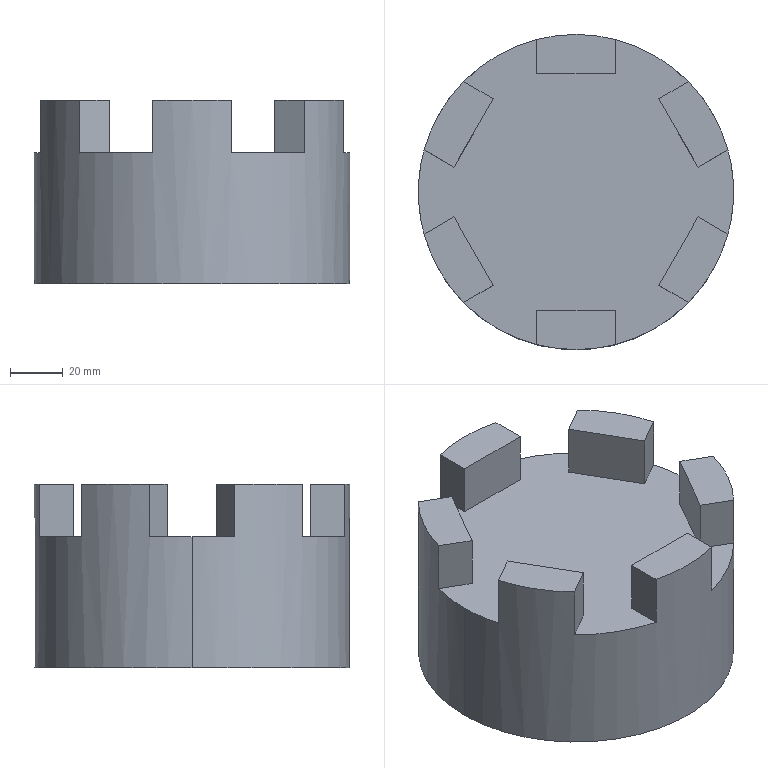Part | SolidWorks | features ICE 3, Extrusion 1 | 1 solid | 35 faces | box 120 x 120 x 70 mm | volume 595667 mm3 | plane 31 | cylinder 4 | commonest cylinder face diameters 30 x2 120 x2
STEP:
#1=CARTESIAN_POINT('',(60.,0.,50.));
#2=VERTEX_POINT('',#1);
#3=CARTESIAN_POINT('',(57.812,16.057,50.));
#4=VERTEX_POINT('',#3);
#5=CARTESIAN_POINT('',(0.,0.,50.));
#6=DIRECTION('',(0.,0.,1.));
#7=DIRECTION('',(1.,0.,0.));
#8=AXIS2_PLACEMENT_3D('',#5,#6,#7);
#9=CIRCLE('',#8,60.);
#10=EDGE_CURVE('',#2,#4,#9,.T.);
#11=ORIENTED_EDGE('',*,*,#10,.F.);
#12=CARTESIAN_POINT('',(60.,0.,0.));
#13=VERTEX_POINT('',#12);
#14=CARTESIAN_POINT('',(60.,0.,50.));
#15=DIRECTION('',(0.,0.,-1.));
#16=VECTOR('',#15,1000.);
#17=LINE('',#14,#16);
#18=EDGE_CURVE('',#2,#13,#17,.T.);
#19=ORIENTED_EDGE('',*,*,#18,.T.);
#20=CARTESIAN_POINT('',(-60.,0.,0.));
#21=VERTEX_POINT('',#20);
#22=CARTESIAN_POINT('',(0.,0.,0.));
#23=DIRECTION('',(0.,0.,1.));
#24=DIRECTION('',(1.,0.,0.));
#25=AXIS2_PLACEMENT_3D('',#22,#23,#24);
#26=CIRCLE('',#25,60.);
#27=EDGE_CURVE('',#13,#21,#26,.T.);
#28=ORIENTED_EDGE('',*,*,#27,.T.);
#29=CARTESIAN_POINT('',(-60.,0.,50.));
#30=VERTEX_POINT('',#29);
#31=CARTESIAN_POINT('',(-60.,0.,50.));
#32=DIRECTION('',(0.,0.,-1.));
#33=VECTOR('',#32,1000.);
#34=LINE('',#31,#33);
#35=EDGE_CURVE('',#30,#21,#34,.T.);
#36=ORIENTED_EDGE('',*,*,#35,.F.);
#37=CARTESIAN_POINT('',(-57.812,16.057,50.));
#38=VERTEX_POINT('',#37);
#39=CARTESIAN_POINT('',(0.,0.,50.));
#40=DIRECTION('',(0.,0.,1.));
#41=DIRECTION('',(1.,0.,0.));
#42=AXIS2_PLACEMENT_3D('',#39,#40,#41);
#43=CIRCLE('',#42,60.);
#44=EDGE_CURVE('',#38,#30,#43,.T.);
#45=ORIENTED_EDGE('',*,*,#44,.F.);
#46=CARTESIAN_POINT('',(-57.812,16.057,70.));
#47=VERTEX_POINT('',#46);
#48=CARTESIAN_POINT('',(-57.812,16.057,70.));
#49=DIRECTION('',(0.,0.,-1.));
#50=VECTOR('',#49,1000.);
#51=LINE('',#48,#50);
#52=EDGE_CURVE('',#47,#38,#51,.T.);
#53=ORIENTED_EDGE('',*,*,#52,.F.);
#54=CARTESIAN_POINT('',(-42.812,42.038,70.));
#55=VERTEX_POINT('',#54);
#56=CARTESIAN_POINT('',(0.,0.,70.));
#57=DIRECTION('',(0.,0.,1.));
#58=DIRECTION('',(1.,0.,0.));
#59=AXIS2_PLACEMENT_3D('',#56,#57,#58);
#60=CIRCLE('',#59,60.);
#61=EDGE_CURVE('',#55,#47,#60,.T.);
#62=ORIENTED_EDGE('',*,*,#61,.F.);
#63=CARTESIAN_POINT('',(-42.812,42.038,50.));
#64=VERTEX_POINT('',#63);
#65=CARTESIAN_POINT('',(-42.812,42.038,70.));
#66=DIRECTION('',(0.,0.,-1.));
#67=VECTOR('',#66,1000.);
#68=LINE('',#65,#67);
#69=EDGE_CURVE('',#55,#64,#68,.T.);
#70=ORIENTED_EDGE('',*,*,#69,.T.);
#71=CARTESIAN_POINT('',(-15.,58.095,50.));
#72=VERTEX_POINT('',#71);
#73=CARTESIAN_POINT('',(0.,0.,50.));
#74=DIRECTION('',(0.,0.,1.));
#75=DIRECTION('',(1.,0.,0.));
#76=AXIS2_PLACEMENT_3D('',#73,#74,#75);
#77=CIRCLE('',#76,60.);
#78=EDGE_CURVE('',#72,#64,#77,.T.);
#79=ORIENTED_EDGE('',*,*,#78,.F.);
#80=CARTESIAN_POINT('',(-15.,58.095,70.));
#81=VERTEX_POINT('',#80);
#82=CARTESIAN_POINT('',(-15.,58.095,70.));
#83=DIRECTION('',(0.,0.,-1.));
#84=VECTOR('',#83,1000.);
#85=LINE('',#82,#84);
#86=EDGE_CURVE('',#81,#72,#85,.T.);
#87=ORIENTED_EDGE('',*,*,#86,.F.);
#88=CARTESIAN_POINT('',(15.,58.095,70.));
#89=VERTEX_POINT('',#88);
#90=CARTESIAN_POINT('',(0.,0.,70.));
#91=DIRECTION('',(0.,0.,1.));
#92=DIRECTION('',(1.,0.,0.));
#93=AXIS2_PLACEMENT_3D('',#90,#91,#92);
#94=CIRCLE('',#93,60.);
#95=EDGE_CURVE('',#89,#81,#94,.T.);
#96=ORIENTED_EDGE('',*,*,#95,.F.);
#97=CARTESIAN_POINT('',(15.,58.095,50.));
#98=VERTEX_POINT('',#97);
#99=CARTESIAN_POINT('',(15.,58.095,70.));
#100=DIRECTION('',(0.,0.,-1.));
#101=VECTOR('',#100,1000.);
#102=LINE('',#99,#101);
#103=EDGE_CURVE('',#89,#98,#102,.T.);
#104=ORIENTED_EDGE('',*,*,#103,.T.);
#105=CARTESIAN_POINT('',(42.812,42.038,50.));
#106=VERTEX_POINT('',#105);
#107=CARTESIAN_POINT('',(0.,0.,50.));
#108=DIRECTION('',(0.,0.,1.));
#109=DIRECTION('',(1.,0.,0.));
#110=AXIS2_PLACEMENT_3D('',#107,#108,#109);
#111=CIRCLE('',#110,60.);
#112=EDGE_CURVE('',#106,#98,#111,.T.);
#113=ORIENTED_EDGE('',*,*,#112,.F.);
#114=CARTESIAN_POINT('',(42.812,42.038,70.));
#115=VERTEX_POINT('',#114);
#116=CARTESIAN_POINT('',(42.812,42.038,70.));
#117=DIRECTION('',(0.,0.,-1.));
#118=VECTOR('',#117,1000.);
#119=LINE('',#116,#118);
#120=EDGE_CURVE('',#115,#106,#119,.T.);
#121=ORIENTED_EDGE('',*,*,#120,.F.);
#122=CARTESIAN_POINT('',(57.812,16.057,70.));
#123=VERTEX_POINT('',#122);
#124=CARTESIAN_POINT('',(0.,0.,70.));
#125=DIRECTION('',(0.,0.,1.));
#126=DIRECTION('',(1.,0.,0.));
#127=AXIS2_PLACEMENT_3D('',#124,#125,#126);
#128=CIRCLE('',#127,60.);
#129=EDGE_CURVE('',#123,#115,#128,.T.);
#130=ORIENTED_EDGE('',*,*,#129,.F.);
#131=CARTESIAN_POINT('',(57.812,16.057,70.));
#132=DIRECTION('',(0.,0.,-1.));
#133=VECTOR('',#132,1000.);
#134=LINE('',#131,#133);
#135=EDGE_CURVE('',#123,#4,#134,.T.);
#136=ORIENTED_EDGE('',*,*,#135,.T.);
#137=EDGE_LOOP('',(#11,#19,#28,#36,#45,#53,#62,#70,#79,#87,#96,#104,#113,#121,#130,#136));
#138=FACE_OUTER_BOUND('',#137,.T.);
#139=CARTESIAN_POINT('',(0.,0.,50.));
#140=DIRECTION('',(0.,0.,-1.));
#141=DIRECTION('',(-1.,0.,0.));
#142=AXIS2_PLACEMENT_3D('',#139,#140,#141);
#143=CYLINDRICAL_SURFACE('',#142,60.);
#144=ADVANCED_FACE('',(#138),#143,.T.);
#145=CARTESIAN_POINT('',(-15.,0.,30.));
#146=VERTEX_POINT('',#145);
#147=CARTESIAN_POINT('',(15.,0.,30.));
#148=VERTEX_POINT('',#147);
#149=CARTESIAN_POINT('',(0.,0.,30.));
#150=DIRECTION('',(0.,0.,1.));
#151=DIRECTION('',(1.,0.,0.));
#152=AXIS2_PLACEMENT_3D('',#149,#150,#151);
#153=CIRCLE('',#152,15.);
#154=EDGE_CURVE('',#146,#148,#153,.T.);
#155=ORIENTED_EDGE('',*,*,#154,.T.);
#156=CARTESIAN_POINT('',(15.,0.,0.));
#157=VERTEX_POINT('',#156);
#158=CARTESIAN_POINT('',(15.,0.,30.));
#159=DIRECTION('',(0.,0.,-1.));
#160=VECTOR('',#159,1000.);
#161=LINE('',#158,#160);
#162=EDGE_CURVE('',#148,#157,#161,.T.);
#163=ORIENTED_EDGE('',*,*,#162,.T.);
#164=CARTESIAN_POINT('',(-15.,0.,0.));
#165=VERTEX_POINT('',#164);
#166=CARTESIAN_POINT('',(0.,0.,0.));
#167=DIRECTION('',(0.,0.,1.));
#168=DIRECTION('',(1.,0.,0.));
#169=AXIS2_PLACEMENT_3D('',#166,#167,#168);
#170=CIRCLE('',#169,15.);
#171=EDGE_CURVE('',#165,#157,#170,.T.);
#172=ORIENTED_EDGE('',*,*,#171,.F.);
#173=CARTESIAN_POINT('',(-15.,0.,30.));
#174=DIRECTION('',(0.,0.,-1.));
#175=VECTOR('',#174,1000.);
#176=LINE('',#173,#175);
#177=EDGE_CURVE('',#146,#165,#176,.T.);
#178=ORIENTED_EDGE('',*,*,#177,.F.);
#179=EDGE_LOOP('',(#155,#163,#172,#178));
#180=FACE_OUTER_BOUND('',#179,.T.);
#181=CARTESIAN_POINT('',(0.,0.,30.));
#182=DIRECTION('',(0.,0.,-1.));
#183=DIRECTION('',(-1.,0.,0.));
#184=AXIS2_PLACEMENT_3D('',#181,#182,#183);
#185=CYLINDRICAL_SURFACE('',#184,15.);
#186=ADVANCED_FACE('',(#180),#185,.F.);
#187=CARTESIAN_POINT('',(0.,0.,0.));
#188=DIRECTION('',(0.,0.,1.));
#189=DIRECTION('',(1.,0.,0.));
#190=AXIS2_PLACEMENT_3D('',#187,#188,#189);
#191=CIRCLE('',#190,60.);
#192=EDGE_CURVE('',#21,#13,#191,.T.);
#193=ORIENTED_EDGE('',*,*,#192,.F.);
#194=ORIENTED_EDGE('',*,*,#27,.F.);
#195=EDGE_LOOP('',(#193,#194));
#196=FACE_OUTER_BOUND('',#195,.T.);
#197=CARTESIAN_POINT('',(-5.,17.,0.));
#198=VERTEX_POINT('',#197);
#199=CARTESIAN_POINT('',(-5.,14.142,0.));
#200=VERTEX_POINT('',#199);
#201=CARTESIAN_POINT('',(-5.,17.,0.));
#202=DIRECTION('',(0.,-1.,0.));
#203=VECTOR('',#202,1000.);
#204=LINE('',#201,#203);
#205=EDGE_CURVE('',#198,#200,#204,.T.);
#206=ORIENTED_EDGE('',*,*,#205,.T.);
#207=CARTESIAN_POINT('',(0.,0.,0.));
#208=DIRECTION('',(0.,0.,1.));
#209=DIRECTION('',(1.,0.,0.));
#210=AXIS2_PLACEMENT_3D('',#207,#208,#209);
#211=CIRCLE('',#210,15.);
#212=EDGE_CURVE('',#200,#165,#211,.T.);
#213=ORIENTED_EDGE('',*,*,#212,.T.);
#214=ORIENTED_EDGE('',*,*,#171,.T.);
#215=CARTESIAN_POINT('',(5.,14.142,0.));
#216=VERTEX_POINT('',#215);
#217=CARTESIAN_POINT('',(0.,0.,0.));
#218=DIRECTION('',(0.,0.,1.));
#219=DIRECTION('',(1.,0.,0.));
#220=AXIS2_PLACEMENT_3D('',#217,#218,#219);
#221=CIRCLE('',#220,15.);
#222=EDGE_CURVE('',#157,#216,#221,.T.);
#223=ORIENTED_EDGE('',*,*,#222,.T.);
#224=CARTESIAN_POINT('',(5.,17.,0.));
#225=VERTEX_POINT('',#224);
#226=CARTESIAN_POINT('',(5.,17.,0.));
#227=DIRECTION('',(0.,-1.,0.));
#228=VECTOR('',#227,1000.);
#229=LINE('',#226,#228);
#230=EDGE_CURVE('',#225,#216,#229,.T.);
#231=ORIENTED_EDGE('',*,*,#230,.F.);
#232=CARTESIAN_POINT('',(5.,17.,0.));
#233=DIRECTION('',(-1.,0.,0.));
#234=VECTOR('',#233,1000.);
#235=LINE('',#232,#234);
#236=EDGE_CURVE('',#225,#198,#235,.T.);
#237=ORIENTED_EDGE('',*,*,#236,.T.);
#238=EDGE_LOOP('',(#206,#213,#214,#223,#231,#237));
#239=FACE_BOUND('',#238,.T.);
#240=CARTESIAN_POINT('',(0.,0.,0.));
#241=DIRECTION('',(0.,0.,1.));
#242=DIRECTION('',(1.,0.,0.));
#243=AXIS2_PLACEMENT_3D('',#240,#241,#242);
#244=PLANE('',#243);
#245=ADVANCED_FACE('',(#196,#239),#244,.F.);
#246=ORIENTED_EDGE('',*,*,#162,.F.);
#247=CARTESIAN_POINT('',(0.,0.,30.));
#248=DIRECTION('',(0.,0.,1.));
#249=DIRECTION('',(1.,0.,0.));
#250=AXIS2_PLACEMENT_3D('',#247,#248,#249);
#251=CIRCLE('',#250,15.);
#252=EDGE_CURVE('',#148,#146,#251,.T.);
#253=ORIENTED_EDGE('',*,*,#252,.T.);
#254=ORIENTED_EDGE('',*,*,#177,.T.);
#255=ORIENTED_EDGE('',*,*,#212,.F.);
#256=CARTESIAN_POINT('',(-5.,14.142,15.));
#257=VERTEX_POINT('',#256);
#258=CARTESIAN_POINT('',(-5.,14.142,30.));
#259=DIRECTION('',(0.,0.,1.));
#260=VECTOR('',#259,1000.);
#261=LINE('',#258,#260);
#262=EDGE_CURVE('',#200,#257,#261,.T.);
#263=ORIENTED_EDGE('',*,*,#262,.T.);
#264=CARTESIAN_POINT('',(5.,14.142,15.));
#265=VERTEX_POINT('',#264);
#266=CARTESIAN_POINT('',(0.,0.,15.));
#267=DIRECTION('',(0.,0.,1.));
#268=DIRECTION('',(1.,0.,0.));
#269=AXIS2_PLACEMENT_3D('',#266,#267,#268);
#270=CIRCLE('',#269,15.);
#271=EDGE_CURVE('',#265,#257,#270,.T.);
#272=ORIENTED_EDGE('',*,*,#271,.F.);
#273=CARTESIAN_POINT('',(5.,14.142,30.));
#274=DIRECTION('',(0.,0.,1.));
#275=VECTOR('',#274,1000.);
#276=LINE('',#273,#275);
#277=EDGE_CURVE('',#216,#265,#276,.T.);
#278=ORIENTED_EDGE('',*,*,#277,.F.);
#279=ORIENTED_EDGE('',*,*,#222,.F.);
#280=EDGE_LOOP('',(#246,#253,#254,#255,#263,#272,#278,#279));
#281=FACE_OUTER_BOUND('',#280,.T.);
#282=CARTESIAN_POINT('',(0.,0.,30.));
#283=DIRECTION('',(0.,0.,-1.));
#284=DIRECTION('',(-1.,0.,0.));
#285=AXIS2_PLACEMENT_3D('',#282,#283,#284);
#286=CYLINDRICAL_SURFACE('',#285,15.);
#287=ADVANCED_FACE('',(#281),#286,.F.);
#288=ORIENTED_EDGE('',*,*,#18,.F.);
#289=CARTESIAN_POINT('',(57.812,-16.057,50.));
#290=VERTEX_POINT('',#289);
#291=CARTESIAN_POINT('',(0.,0.,50.));
#292=DIRECTION('',(0.,0.,1.));
#293=DIRECTION('',(1.,0.,0.));
#294=AXIS2_PLACEMENT_3D('',#291,#292,#293);
#295=CIRCLE('',#294,60.);
#296=EDGE_CURVE('',#290,#2,#295,.T.);
#297=ORIENTED_EDGE('',*,*,#296,.F.);
#298=CARTESIAN_POINT('',(57.812,-16.057,70.));
#299=VERTEX_POINT('',#298);
#300=CARTESIAN_POINT('',(57.812,-16.057,70.));
#301=DIRECTION('',(0.,0.,-1.));
#302=VECTOR('',#301,1000.);
#303=LINE('',#300,#302);
#304=EDGE_CURVE('',#299,#290,#303,.T.);
#305=ORIENTED_EDGE('',*,*,#304,.F.);
#306=CARTESIAN_POINT('',(42.812,-42.038,70.));
#307=VERTEX_POINT('',#306);
#308=CARTESIAN_POINT('',(0.,0.,70.));
#309=DIRECTION('',(0.,0.,1.));
#310=DIRECTION('',(1.,0.,0.));
#311=AXIS2_PLACEMENT_3D('',#308,#309,#310);
#312=CIRCLE('',#311,60.);
#313=EDGE_CURVE('',#307,#299,#312,.T.);
#314=ORIENTED_EDGE('',*,*,#313,.F.);
#315=CARTESIAN_POINT('',(42.812,-42.038,50.));
#316=VERTEX_POINT('',#315);
#317=CARTESIAN_POINT('',(42.812,-42.038,70.));
#318=DIRECTION('',(0.,0.,-1.));
#319=VECTOR('',#318,1000.);
#320=LINE('',#317,#319);
#321=EDGE_CURVE('',#307,#316,#320,.T.);
#322=ORIENTED_EDGE('',*,*,#321,.T.);
#323=CARTESIAN_POINT('',(15.,-58.095,50.));
#324=VERTEX_POINT('',#323);
#325=CARTESIAN_POINT('',(0.,0.,50.));
#326=DIRECTION('',(0.,0.,1.));
#327=DIRECTION('',(1.,0.,0.));
#328=AXIS2_PLACEMENT_3D('',#325,#326,#327);
#329=CIRCLE('',#328,60.);
#330=EDGE_CURVE('',#324,#316,#329,.T.);
#331=ORIENTED_EDGE('',*,*,#330,.F.);
#332=CARTESIAN_POINT('',(15.,-58.095,70.));
#333=VERTEX_POINT('',#332);
#334=CARTESIAN_POINT('',(15.,-58.095,70.));
#335=DIRECTION('',(0.,0.,-1.));
#336=VECTOR('',#335,1000.);
#337=LINE('',#334,#336);
#338=EDGE_CURVE('',#333,#324,#337,.T.);
#339=ORIENTED_EDGE('',*,*,#338,.F.);
#340=CARTESIAN_POINT('',(-15.,-58.095,70.));
#341=VERTEX_POINT('',#340);
#342=CARTESIAN_POINT('',(0.,0.,70.));
#343=DIRECTION('',(0.,0.,1.));
#344=DIRECTION('',(1.,0.,0.));
#345=AXIS2_PLACEMENT_3D('',#342,#343,#344);
#346=CIRCLE('',#345,60.);
#347=EDGE_CURVE('',#341,#333,#346,.T.);
#348=ORIENTED_EDGE('',*,*,#347,.F.);
#349=CARTESIAN_POINT('',(-15.,-58.095,50.));
#350=VERTEX_POINT('',#349);
#351=CARTESIAN_POINT('',(-15.,-58.095,70.));
#352=DIRECTION('',(0.,0.,-1.));
#353=VECTOR('',#352,1000.);
#354=LINE('',#351,#353);
#355=EDGE_CURVE('',#341,#350,#354,.T.);
#356=ORIENTED_EDGE('',*,*,#355,.T.);
#357=CARTESIAN_POINT('',(-42.812,-42.038,50.));
#358=VERTEX_POINT('',#357);
#359=CARTESIAN_POINT('',(0.,0.,50.));
#360=DIRECTION('',(0.,0.,1.));
#361=DIRECTION('',(1.,0.,0.));
#362=AXIS2_PLACEMENT_3D('',#359,#360,#361);
#363=CIRCLE('',#362,60.);
#364=EDGE_CURVE('',#358,#350,#363,.T.);
#365=ORIENTED_EDGE('',*,*,#364,.F.);
#366=CARTESIAN_POINT('',(-42.812,-42.038,70.));
#367=VERTEX_POINT('',#366);
#368=CARTESIAN_POINT('',(-42.812,-42.038,70.));
#369=DIRECTION('',(0.,0.,-1.));
#370=VECTOR('',#369,1000.);
#371=LINE('',#368,#370);
#372=EDGE_CURVE('',#367,#358,#371,.T.);
#373=ORIENTED_EDGE('',*,*,#372,.F.);
#374=CARTESIAN_POINT('',(-57.812,-16.057,70.));
#375=VERTEX_POINT('',#374);
#376=CARTESIAN_POINT('',(0.,0.,70.));
#377=DIRECTION('',(0.,0.,1.));
#378=DIRECTION('',(1.,0.,0.));
#379=AXIS2_PLACEMENT_3D('',#376,#377,#378);
#380=CIRCLE('',#379,60.);
#381=EDGE_CURVE('',#375,#367,#380,.T.);
#382=ORIENTED_EDGE('',*,*,#381,.F.);
#383=CARTESIAN_POINT('',(-57.812,-16.057,50.));
#384=VERTEX_POINT('',#383);
#385=CARTESIAN_POINT('',(-57.812,-16.057,70.));
#386=DIRECTION('',(0.,0.,-1.));
#387=VECTOR('',#386,1000.);
#388=LINE('',#385,#387);
#389=EDGE_CURVE('',#375,#384,#388,.T.);
#390=ORIENTED_EDGE('',*,*,#389,.T.);
#391=CARTESIAN_POINT('',(0.,0.,50.));
#392=DIRECTION('',(0.,0.,1.));
#393=DIRECTION('',(1.,0.,0.));
#394=AXIS2_PLACEMENT_3D('',#391,#392,#393);
#395=CIRCLE('',#394,60.);
#396=EDGE_CURVE('',#30,#384,#395,.T.);
#397=ORIENTED_EDGE('',*,*,#396,.F.);
#398=ORIENTED_EDGE('',*,*,#35,.T.);
#399=ORIENTED_EDGE('',*,*,#192,.T.);
#400=EDGE_LOOP('',(#288,#297,#305,#314,#322,#331,#339,#348,#356,#365,#373,#382,#390,#397,#398,#399));
#401=FACE_OUTER_BOUND('',#400,.T.);
#402=CARTESIAN_POINT('',(0.,0.,50.));
#403=DIRECTION('',(0.,0.,-1.));
#404=DIRECTION('',(-1.,0.,0.));
#405=AXIS2_PLACEMENT_3D('',#402,#403,#404);
#406=CYLINDRICAL_SURFACE('',#405,60.);
#407=ADVANCED_FACE('',(#401),#406,.T.);
#408=CARTESIAN_POINT('',(15.,45.,50.));
#409=VERTEX_POINT('',#408);
#410=CARTESIAN_POINT('',(15.,58.095,50.));
#411=DIRECTION('',(0.,1.,0.));
#412=VECTOR('',#411,1000.);
#413=LINE('',#410,#412);
#414=EDGE_CURVE('',#409,#98,#413,.T.);
#415=ORIENTED_EDGE('',*,*,#414,.F.);
#416=CARTESIAN_POINT('',(-15.,45.,50.));
#417=VERTEX_POINT('',#416);
#418=CARTESIAN_POINT('',(-15.,45.,50.));
#419=DIRECTION('',(1.,0.,0.));
#420=VECTOR('',#419,1000.);
#421=LINE('',#418,#420);
#422=EDGE_CURVE('',#417,#409,#421,.T.);
#423=ORIENTED_EDGE('',*,*,#422,.F.);
#424=CARTESIAN_POINT('',(-15.,58.095,50.));
#425=DIRECTION('',(0.,-1.,0.));
#426=VECTOR('',#425,1000.);
#427=LINE('',#424,#426);
#428=EDGE_CURVE('',#72,#417,#427,.T.);
#429=ORIENTED_EDGE('',*,*,#428,.F.);
#430=ORIENTED_EDGE('',*,*,#78,.T.);
#431=CARTESIAN_POINT('',(-31.471,35.49,50.));
#432=VERTEX_POINT('',#431);
#433=CARTESIAN_POINT('',(-42.812,42.038,50.));
#434=DIRECTION('',(-0.866,0.5,0.));
#435=VECTOR('',#434,1000.);
#436=LINE('',#433,#435);
#437=EDGE_CURVE('',#432,#64,#436,.T.);
#438=ORIENTED_EDGE('',*,*,#437,.F.);
#439=CARTESIAN_POINT('',(-46.471,9.51,50.));
#440=VERTEX_POINT('',#439);
#441=CARTESIAN_POINT('',(-46.471,9.51,50.));
#442=DIRECTION('',(0.5,0.866,0.));
#443=VECTOR('',#442,1000.);
#444=LINE('',#441,#443);
#445=EDGE_CURVE('',#440,#432,#444,.T.);
#446=ORIENTED_EDGE('',*,*,#445,.F.);
#447=CARTESIAN_POINT('',(-57.812,16.057,50.));
#448=DIRECTION('',(0.866,-0.5,0.));
#449=VECTOR('',#448,1000.);
#450=LINE('',#447,#449);
#451=EDGE_CURVE('',#38,#440,#450,.T.);
#452=ORIENTED_EDGE('',*,*,#451,.F.);
#453=ORIENTED_EDGE('',*,*,#44,.T.);
#454=ORIENTED_EDGE('',*,*,#396,.T.);
#455=CARTESIAN_POINT('',(-46.471,-9.51,50.));
#456=VERTEX_POINT('',#455);
#457=CARTESIAN_POINT('',(-57.812,-16.057,50.));
#458=DIRECTION('',(-0.866,-0.5,0.));
#459=VECTOR('',#458,1000.);
#460=LINE('',#457,#459);
#461=EDGE_CURVE('',#456,#384,#460,.T.);
#462=ORIENTED_EDGE('',*,*,#461,.F.);
#463=CARTESIAN_POINT('',(-31.471,-35.49,50.));
#464=VERTEX_POINT('',#463);
#465=CARTESIAN_POINT('',(-31.471,-35.49,50.));
#466=DIRECTION('',(-0.5,0.866,0.));
#467=VECTOR('',#466,1000.);
#468=LINE('',#465,#467);
#469=EDGE_CURVE('',#464,#456,#468,.T.);
#470=ORIENTED_EDGE('',*,*,#469,.F.);
#471=CARTESIAN_POINT('',(-42.812,-42.038,50.));
#472=DIRECTION('',(0.866,0.5,0.));
#473=VECTOR('',#472,1000.);
#474=LINE('',#471,#473);
#475=EDGE_CURVE('',#358,#464,#474,.T.);
#476=ORIENTED_EDGE('',*,*,#475,.F.);
#477=ORIENTED_EDGE('',*,*,#364,.T.);
#478=CARTESIAN_POINT('',(-15.,-45.,50.));
#479=VERTEX_POINT('',#478);
#480=CARTESIAN_POINT('',(-15.,-58.095,50.));
#481=DIRECTION('',(0.,-1.,0.));
#482=VECTOR('',#481,1000.);
#483=LINE('',#480,#482);
#484=EDGE_CURVE('',#479,#350,#483,.T.);
#485=ORIENTED_EDGE('',*,*,#484,.F.);
#486=CARTESIAN_POINT('',(15.,-45.,50.));
#487=VERTEX_POINT('',#486);
#488=CARTESIAN_POINT('',(15.,-45.,50.));
#489=DIRECTION('',(-1.,0.,0.));
#490=VECTOR('',#489,1000.);
#491=LINE('',#488,#490);
#492=EDGE_CURVE('',#487,#479,#491,.T.);
#493=ORIENTED_EDGE('',*,*,#492,.F.);
#494=CARTESIAN_POINT('',(15.,-58.095,50.));
#495=DIRECTION('',(0.,1.,0.));
#496=VECTOR('',#495,1000.);
#497=LINE('',#494,#496);
#498=EDGE_CURVE('',#324,#487,#497,.T.);
#499=ORIENTED_EDGE('',*,*,#498,.F.);
#500=ORIENTED_EDGE('',*,*,#330,.T.);
#501=CARTESIAN_POINT('',(31.471,-35.49,50.));
#502=VERTEX_POINT('',#501);
#503=CARTESIAN_POINT('',(42.812,-42.038,50.));
#504=DIRECTION('',(0.866,-0.5,0.));
#505=VECTOR('',#504,1000.);
#506=LINE('',#503,#505);
#507=EDGE_CURVE('',#502,#316,#506,.T.);
#508=ORIENTED_EDGE('',*,*,#507,.F.);
#509=CARTESIAN_POINT('',(46.471,-9.51,50.));
#510=VERTEX_POINT('',#509);
#511=CARTESIAN_POINT('',(46.471,-9.51,50.));
#512=DIRECTION('',(-0.5,-0.866,0.));
#513=VECTOR('',#512,1000.);
#514=LINE('',#511,#513);
#515=EDGE_CURVE('',#510,#502,#514,.T.);
#516=ORIENTED_EDGE('',*,*,#515,.F.);
#517=CARTESIAN_POINT('',(57.812,-16.057,50.));
#518=DIRECTION('',(-0.866,0.5,0.));
#519=VECTOR('',#518,1000.);
#520=LINE('',#517,#519);
#521=EDGE_CURVE('',#290,#510,#520,.T.);
#522=ORIENTED_EDGE('',*,*,#521,.F.);
#523=ORIENTED_EDGE('',*,*,#296,.T.);
#524=ORIENTED_EDGE('',*,*,#10,.T.);
#525=CARTESIAN_POINT('',(46.471,9.51,50.));
#526=VERTEX_POINT('',#525);
#527=CARTESIAN_POINT('',(57.812,16.057,50.));
#528=DIRECTION('',(0.866,0.5,0.));
#529=VECTOR('',#528,1000.);
#530=LINE('',#527,#529);
#531=EDGE_CURVE('',#526,#4,#530,.T.);
#532=ORIENTED_EDGE('',*,*,#531,.F.);
#533=CARTESIAN_POINT('',(31.471,35.49,50.));
#534=VERTEX_POINT('',#533);
#535=CARTESIAN_POINT('',(31.471,35.49,50.));
#536=DIRECTION('',(0.5,-0.866,0.));
#537=VECTOR('',#536,1000.);
#538=LINE('',#535,#537);
#539=EDGE_CURVE('',#534,#526,#538,.T.);
#540=ORIENTED_EDGE('',*,*,#539,.F.);
#541=CARTESIAN_POINT('',(42.812,42.038,50.));
#542=DIRECTION('',(-0.866,-0.5,0.));
#543=VECTOR('',#542,1000.);
#544=LINE('',#541,#543);
#545=EDGE_CURVE('',#106,#534,#544,.T.);
#546=ORIENTED_EDGE('',*,*,#545,.F.);
#547=ORIENTED_EDGE('',*,*,#112,.T.);
#548=EDGE_LOOP('',(#415,#423,#429,#430,#438,#446,#452,#453,#454,#462,#470,#476,#477,#485,#493,#499,#500,#508,#516,#522,#523,#524,#532,#540,#546,#547));
#549=FACE_OUTER_BOUND('',#548,.T.);
#550=CARTESIAN_POINT('',(0.,0.,50.));
#551=DIRECTION('',(0.,0.,1.));
#552=DIRECTION('',(1.,0.,0.));
#553=AXIS2_PLACEMENT_3D('',#550,#551,#552);
#554=PLANE('',#553);
#555=ADVANCED_FACE('',(#549),#554,.T.);
#556=ORIENTED_EDGE('',*,*,#154,.F.);
#557=ORIENTED_EDGE('',*,*,#252,.F.);
#558=EDGE_LOOP('',(#556,#557));
#559=FACE_OUTER_BOUND('',#558,.T.);
#560=CARTESIAN_POINT('',(0.,0.,30.));
#561=DIRECTION('',(0.,0.,1.));
#562=DIRECTION('',(1.,0.,0.));
#563=AXIS2_PLACEMENT_3D('',#560,#561,#562);
#564=PLANE('',#563);
#565=ADVANCED_FACE('',(#559),#564,.F.);
#566=ORIENTED_EDGE('',*,*,#545,.T.);
#567=CARTESIAN_POINT('',(31.471,35.49,70.));
#568=VERTEX_POINT('',#567);
#569=CARTESIAN_POINT('',(31.471,35.49,70.));
#570=DIRECTION('',(0.,0.,-1.));
#571=VECTOR('',#570,1000.);
#572=LINE('',#569,#571);
#573=EDGE_CURVE('',#568,#534,#572,.T.);
#574=ORIENTED_EDGE('',*,*,#573,.F.);
#575=CARTESIAN_POINT('',(42.812,42.038,70.));
#576=DIRECTION('',(-0.866,-0.5,0.));
#577=VECTOR('',#576,1000.);
#578=LINE('',#575,#577);
#579=EDGE_CURVE('',#115,#568,#578,.T.);
#580=ORIENTED_EDGE('',*,*,#579,.F.);
#581=ORIENTED_EDGE('',*,*,#120,.T.);
#582=EDGE_LOOP('',(#566,#574,#580,#581));
#583=FACE_OUTER_BOUND('',#582,.T.);
#584=CARTESIAN_POINT('',(42.812,42.038,70.));
#585=DIRECTION('',(0.5,-0.866,0.));
#586=DIRECTION('',(0.866,0.5,0.));
#587=AXIS2_PLACEMENT_3D('',#584,#585,#586);
#588=PLANE('',#587);
#589=ADVANCED_FACE('',(#583),#588,.F.);
#590=ORIENTED_EDGE('',*,*,#539,.T.);
#591=CARTESIAN_POINT('',(46.471,9.51,70.));
#592=VERTEX_POINT('',#591);
#593=CARTESIAN_POINT('',(46.471,9.51,70.));
#594=DIRECTION('',(0.,0.,-1.));
#595=VECTOR('',#594,1000.);
#596=LINE('',#593,#595);
#597=EDGE_CURVE('',#592,#526,#596,.T.);
#598=ORIENTED_EDGE('',*,*,#597,.F.);
#599=CARTESIAN_POINT('',(31.471,35.49,70.));
#600=DIRECTION('',(0.5,-0.866,0.));
#601=VECTOR('',#600,1000.);
#602=LINE('',#599,#601);
#603=EDGE_CURVE('',#568,#592,#602,.T.);
#604=ORIENTED_EDGE('',*,*,#603,.F.);
#605=ORIENTED_EDGE('',*,*,#573,.T.);
#606=EDGE_LOOP('',(#590,#598,#604,#605));
#607=FACE_OUTER_BOUND('',#606,.T.);
#608=CARTESIAN_POINT('',(31.471,35.49,70.));
#609=DIRECTION('',(0.866,0.5,0.));
#610=DIRECTION('',(-0.5,0.866,0.));
#611=AXIS2_PLACEMENT_3D('',#608,#609,#610);
#612=PLANE('',#611);
#613=ADVANCED_FACE('',(#607),#612,.F.);
#614=ORIENTED_EDGE('',*,*,#531,.T.);
#615=ORIENTED_EDGE('',*,*,#135,.F.);
#616=CARTESIAN_POINT('',(57.812,16.057,70.));
#617=DIRECTION('',(0.866,0.5,0.));
#618=VECTOR('',#617,1000.);
#619=LINE('',#616,#618);
#620=EDGE_CURVE('',#592,#123,#619,.T.);
#621=ORIENTED_EDGE('',*,*,#620,.F.);
#622=ORIENTED_EDGE('',*,*,#597,.T.);
#623=EDGE_LOOP('',(#614,#615,#621,#622));
#624=FACE_OUTER_BOUND('',#623,.T.);
#625=CARTESIAN_POINT('',(57.812,16.057,70.));
#626=DIRECTION('',(-0.5,0.866,0.));
#627=DIRECTION('',(-0.866,-0.5,0.));
#628=AXIS2_PLACEMENT_3D('',#625,#626,#627);
#629=PLANE('',#628);
#630=ADVANCED_FACE('',(#624),#629,.F.);
#631=ORIENTED_EDGE('',*,*,#129,.T.);
#632=ORIENTED_EDGE('',*,*,#579,.T.);
#633=ORIENTED_EDGE('',*,*,#603,.T.);
#634=ORIENTED_EDGE('',*,*,#620,.T.);
#635=EDGE_LOOP('',(#631,#632,#633,#634));
#636=FACE_OUTER_BOUND('',#635,.T.);
#637=CARTESIAN_POINT('',(0.,0.,70.));
#638=DIRECTION('',(0.,0.,1.));
#639=DIRECTION('',(1.,0.,0.));
#640=AXIS2_PLACEMENT_3D('',#637,#638,#639);
#641=PLANE('',#640);
#642=ADVANCED_FACE('',(#636),#641,.T.);
#643=ORIENTED_EDGE('',*,*,#521,.T.);
#644=CARTESIAN_POINT('',(46.471,-9.51,70.));
#645=VERTEX_POINT('',#644);
#646=CARTESIAN_POINT('',(46.471,-9.51,70.));
#647=DIRECTION('',(0.,0.,-1.));
#648=VECTOR('',#647,1000.);
#649=LINE('',#646,#648);
#650=EDGE_CURVE('',#645,#510,#649,.T.);
#651=ORIENTED_EDGE('',*,*,#650,.F.);
#652=CARTESIAN_POINT('',(57.812,-16.057,70.));
#653=DIRECTION('',(-0.866,0.5,0.));
#654=VECTOR('',#653,1000.);
#655=LINE('',#652,#654);
#656=EDGE_CURVE('',#299,#645,#655,.T.);
#657=ORIENTED_EDGE('',*,*,#656,.F.);
#658=ORIENTED_EDGE('',*,*,#304,.T.);
#659=EDGE_LOOP('',(#643,#651,#657,#658));
#660=FACE_OUTER_BOUND('',#659,.T.);
#661=CARTESIAN_POINT('',(57.812,-16.057,70.));
#662=DIRECTION('',(-0.5,-0.866,0.));
#663=DIRECTION('',(0.866,-0.5,0.));
#664=AXIS2_PLACEMENT_3D('',#661,#662,#663);
#665=PLANE('',#664);
#666=ADVANCED_FACE('',(#660),#665,.F.);
#667=ORIENTED_EDGE('',*,*,#515,.T.);
#668=CARTESIAN_POINT('',(31.471,-35.49,70.));
#669=VERTEX_POINT('',#668);
#670=CARTESIAN_POINT('',(31.471,-35.49,70.));
#671=DIRECTION('',(0.,0.,-1.));
#672=VECTOR('',#671,1000.);
#673=LINE('',#670,#672);
#674=EDGE_CURVE('',#669,#502,#673,.T.);
#675=ORIENTED_EDGE('',*,*,#674,.F.);
#676=CARTESIAN_POINT('',(46.471,-9.51,70.));
#677=DIRECTION('',(-0.5,-0.866,0.));
#678=VECTOR('',#677,1000.);
#679=LINE('',#676,#678);
#680=EDGE_CURVE('',#645,#669,#679,.T.);
#681=ORIENTED_EDGE('',*,*,#680,.F.);
#682=ORIENTED_EDGE('',*,*,#650,.T.);
#683=EDGE_LOOP('',(#667,#675,#681,#682));
#684=FACE_OUTER_BOUND('',#683,.T.);
#685=CARTESIAN_POINT('',(46.471,-9.51,70.));
#686=DIRECTION('',(0.866,-0.5,0.));
#687=DIRECTION('',(0.5,0.866,0.));
#688=AXIS2_PLACEMENT_3D('',#685,#686,#687);
#689=PLANE('',#688);
#690=ADVANCED_FACE('',(#684),#689,.F.);
#691=ORIENTED_EDGE('',*,*,#507,.T.);
#692=ORIENTED_EDGE('',*,*,#321,.F.);
#693=CARTESIAN_POINT('',(42.812,-42.038,70.));
#694=DIRECTION('',(0.866,-0.5,0.));
#695=VECTOR('',#694,1000.);
#696=LINE('',#693,#695);
#697=EDGE_CURVE('',#669,#307,#696,.T.);
#698=ORIENTED_EDGE('',*,*,#697,.F.);
#699=ORIENTED_EDGE('',*,*,#674,.T.);
#700=EDGE_LOOP('',(#691,#692,#698,#699));
#701=FACE_OUTER_BOUND('',#700,.T.);
#702=CARTESIAN_POINT('',(42.812,-42.038,70.));
#703=DIRECTION('',(0.5,0.866,0.));
#704=DIRECTION('',(-0.866,0.5,0.));
#705=AXIS2_PLACEMENT_3D('',#702,#703,#704);
#706=PLANE('',#705);
#707=ADVANCED_FACE('',(#701),#706,.F.);
#708=ORIENTED_EDGE('',*,*,#313,.T.);
#709=ORIENTED_EDGE('',*,*,#656,.T.);
#710=ORIENTED_EDGE('',*,*,#680,.T.);
#711=ORIENTED_EDGE('',*,*,#697,.T.);
#712=EDGE_LOOP('',(#708,#709,#710,#711));
#713=FACE_OUTER_BOUND('',#712,.T.);
#714=CARTESIAN_POINT('',(0.,0.,70.));
#715=DIRECTION('',(0.,0.,1.));
#716=DIRECTION('',(1.,0.,0.));
#717=AXIS2_PLACEMENT_3D('',#714,#715,#716);
#718=PLANE('',#717);
#719=ADVANCED_FACE('',(#713),#718,.T.);
#720=ORIENTED_EDGE('',*,*,#498,.T.);
#721=CARTESIAN_POINT('',(15.,-45.,70.));
#722=VERTEX_POINT('',#721);
#723=CARTESIAN_POINT('',(15.,-45.,70.));
#724=DIRECTION('',(0.,0.,-1.));
#725=VECTOR('',#724,1000.);
#726=LINE('',#723,#725);
#727=EDGE_CURVE('',#722,#487,#726,.T.);
#728=ORIENTED_EDGE('',*,*,#727,.F.);
#729=CARTESIAN_POINT('',(15.,-58.095,70.));
#730=DIRECTION('',(0.,1.,0.));
#731=VECTOR('',#730,1000.);
#732=LINE('',#729,#731);
#733=EDGE_CURVE('',#333,#722,#732,.T.);
#734=ORIENTED_EDGE('',*,*,#733,.F.);
#735=ORIENTED_EDGE('',*,*,#338,.T.);
#736=EDGE_LOOP('',(#720,#728,#734,#735));
#737=FACE_OUTER_BOUND('',#736,.T.);
#738=CARTESIAN_POINT('',(15.,-58.095,70.));
#739=DIRECTION('',(-1.,0.,0.));
#740=DIRECTION('',(0.,-1.,0.));
#741=AXIS2_PLACEMENT_3D('',#738,#739,#740);
#742=PLANE('',#741);
#743=ADVANCED_FACE('',(#737),#742,.F.);
#744=ORIENTED_EDGE('',*,*,#492,.T.);
#745=CARTESIAN_POINT('',(-15.,-45.,70.));
#746=VERTEX_POINT('',#745);
#747=CARTESIAN_POINT('',(-15.,-45.,70.));
#748=DIRECTION('',(0.,0.,-1.));
#749=VECTOR('',#748,1000.);
#750=LINE('',#747,#749);
#751=EDGE_CURVE('',#746,#479,#750,.T.);
#752=ORIENTED_EDGE('',*,*,#751,.F.);
#753=CARTESIAN_POINT('',(15.,-45.,70.));
#754=DIRECTION('',(-1.,0.,0.));
#755=VECTOR('',#754,1000.);
#756=LINE('',#753,#755);
#757=EDGE_CURVE('',#722,#746,#756,.T.);
#758=ORIENTED_EDGE('',*,*,#757,.F.);
#759=ORIENTED_EDGE('',*,*,#727,.T.);
#760=EDGE_LOOP('',(#744,#752,#758,#759));
#761=FACE_OUTER_BOUND('',#760,.T.);
#762=CARTESIAN_POINT('',(15.,-45.,70.));
#763=DIRECTION('',(0.,-1.,0.));
#764=DIRECTION('',(1.,0.,0.));
#765=AXIS2_PLACEMENT_3D('',#762,#763,#764);
#766=PLANE('',#765);
#767=ADVANCED_FACE('',(#761),#766,.F.);
#768=ORIENTED_EDGE('',*,*,#484,.T.);
#769=ORIENTED_EDGE('',*,*,#355,.F.);
#770=CARTESIAN_POINT('',(-15.,-58.095,70.));
#771=DIRECTION('',(0.,-1.,0.));
#772=VECTOR('',#771,1000.);
#773=LINE('',#770,#772);
#774=EDGE_CURVE('',#746,#341,#773,.T.);
#775=ORIENTED_EDGE('',*,*,#774,.F.);
#776=ORIENTED_EDGE('',*,*,#751,.T.);
#777=EDGE_LOOP('',(#768,#769,#775,#776));
#778=FACE_OUTER_BOUND('',#777,.T.);
#779=CARTESIAN_POINT('',(-15.,-58.095,70.));
#780=DIRECTION('',(1.,0.,0.));
#781=DIRECTION('',(0.,1.,0.));
#782=AXIS2_PLACEMENT_3D('',#779,#780,#781);
#783=PLANE('',#782);
#784=ADVANCED_FACE('',(#778),#783,.F.);
#785=ORIENTED_EDGE('',*,*,#347,.T.);
#786=ORIENTED_EDGE('',*,*,#733,.T.);
#787=ORIENTED_EDGE('',*,*,#757,.T.);
#788=ORIENTED_EDGE('',*,*,#774,.T.);
#789=EDGE_LOOP('',(#785,#786,#787,#788));
#790=FACE_OUTER_BOUND('',#789,.T.);
#791=CARTESIAN_POINT('',(0.,0.,70.));
#792=DIRECTION('',(0.,0.,1.));
#793=DIRECTION('',(1.,0.,0.));
#794=AXIS2_PLACEMENT_3D('',#791,#792,#793);
#795=PLANE('',#794);
#796=ADVANCED_FACE('',(#790),#795,.T.);
#797=ORIENTED_EDGE('',*,*,#475,.T.);
#798=CARTESIAN_POINT('',(-31.471,-35.49,70.));
#799=VERTEX_POINT('',#798);
#800=CARTESIAN_POINT('',(-31.471,-35.49,70.));
#801=DIRECTION('',(0.,0.,-1.));
#802=VECTOR('',#801,1000.);
#803=LINE('',#800,#802);
#804=EDGE_CURVE('',#799,#464,#803,.T.);
#805=ORIENTED_EDGE('',*,*,#804,.F.);
#806=CARTESIAN_POINT('',(-42.812,-42.038,70.));
#807=DIRECTION('',(0.866,0.5,0.));
#808=VECTOR('',#807,1000.);
#809=LINE('',#806,#808);
#810=EDGE_CURVE('',#367,#799,#809,.T.);
#811=ORIENTED_EDGE('',*,*,#810,.F.);
#812=ORIENTED_EDGE('',*,*,#372,.T.);
#813=EDGE_LOOP('',(#797,#805,#811,#812));
#814=FACE_OUTER_BOUND('',#813,.T.);
#815=CARTESIAN_POINT('',(-42.812,-42.038,70.));
#816=DIRECTION('',(-0.5,0.866,0.));
#817=DIRECTION('',(-0.866,-0.5,0.));
#818=AXIS2_PLACEMENT_3D('',#815,#816,#817);
#819=PLANE('',#818);
#820=ADVANCED_FACE('',(#814),#819,.F.);
#821=ORIENTED_EDGE('',*,*,#469,.T.);
#822=CARTESIAN_POINT('',(-46.471,-9.51,70.));
#823=VERTEX_POINT('',#822);
#824=CARTESIAN_POINT('',(-46.471,-9.51,70.));
#825=DIRECTION('',(0.,0.,-1.));
#826=VECTOR('',#825,1000.);
#827=LINE('',#824,#826);
#828=EDGE_CURVE('',#823,#456,#827,.T.);
#829=ORIENTED_EDGE('',*,*,#828,.F.);
#830=CARTESIAN_POINT('',(-31.471,-35.49,70.));
#831=DIRECTION('',(-0.5,0.866,0.));
#832=VECTOR('',#831,1000.);
#833=LINE('',#830,#832);
#834=EDGE_CURVE('',#799,#823,#833,.T.);
#835=ORIENTED_EDGE('',*,*,#834,.F.);
#836=ORIENTED_EDGE('',*,*,#804,.T.);
#837=EDGE_LOOP('',(#821,#829,#835,#836));
#838=FACE_OUTER_BOUND('',#837,.T.);
#839=CARTESIAN_POINT('',(-31.471,-35.49,70.));
#840=DIRECTION('',(-0.866,-0.5,0.));
#841=DIRECTION('',(0.5,-0.866,0.));
#842=AXIS2_PLACEMENT_3D('',#839,#840,#841);
#843=PLANE('',#842);
#844=ADVANCED_FACE('',(#838),#843,.F.);
#845=ORIENTED_EDGE('',*,*,#461,.T.);
#846=ORIENTED_EDGE('',*,*,#389,.F.);
#847=CARTESIAN_POINT('',(-57.812,-16.057,70.));
#848=DIRECTION('',(-0.866,-0.5,0.));
#849=VECTOR('',#848,1000.);
#850=LINE('',#847,#849);
#851=EDGE_CURVE('',#823,#375,#850,.T.);
#852=ORIENTED_EDGE('',*,*,#851,.F.);
#853=ORIENTED_EDGE('',*,*,#828,.T.);
#854=EDGE_LOOP('',(#845,#846,#852,#853));
#855=FACE_OUTER_BOUND('',#854,.T.);
#856=CARTESIAN_POINT('',(-57.812,-16.057,70.));
#857=DIRECTION('',(0.5,-0.866,0.));
#858=DIRECTION('',(0.866,0.5,0.));
#859=AXIS2_PLACEMENT_3D('',#856,#857,#858);
#860=PLANE('',#859);
#861=ADVANCED_FACE('',(#855),#860,.F.);
#862=ORIENTED_EDGE('',*,*,#381,.T.);
#863=ORIENTED_EDGE('',*,*,#810,.T.);
#864=ORIENTED_EDGE('',*,*,#834,.T.);
#865=ORIENTED_EDGE('',*,*,#851,.T.);
#866=EDGE_LOOP('',(#862,#863,#864,#865));
#867=FACE_OUTER_BOUND('',#866,.T.);
#868=CARTESIAN_POINT('',(0.,0.,70.));
#869=DIRECTION('',(0.,0.,1.));
#870=DIRECTION('',(1.,0.,0.));
#871=AXIS2_PLACEMENT_3D('',#868,#869,#870);
#872=PLANE('',#871);
#873=ADVANCED_FACE('',(#867),#872,.T.);
#874=ORIENTED_EDGE('',*,*,#451,.T.);
#875=CARTESIAN_POINT('',(-46.471,9.51,70.));
#876=VERTEX_POINT('',#875);
#877=CARTESIAN_POINT('',(-46.471,9.51,70.));
#878=DIRECTION('',(0.,0.,-1.));
#879=VECTOR('',#878,1000.);
#880=LINE('',#877,#879);
#881=EDGE_CURVE('',#876,#440,#880,.T.);
#882=ORIENTED_EDGE('',*,*,#881,.F.);
#883=CARTESIAN_POINT('',(-57.812,16.057,70.));
#884=DIRECTION('',(0.866,-0.5,0.));
#885=VECTOR('',#884,1000.);
#886=LINE('',#883,#885);
#887=EDGE_CURVE('',#47,#876,#886,.T.);
#888=ORIENTED_EDGE('',*,*,#887,.F.);
#889=ORIENTED_EDGE('',*,*,#52,.T.);
#890=EDGE_LOOP('',(#874,#882,#888,#889));
#891=FACE_OUTER_BOUND('',#890,.T.);
#892=CARTESIAN_POINT('',(-57.812,16.057,70.));
#893=DIRECTION('',(0.5,0.866,0.));
#894=DIRECTION('',(-0.866,0.5,0.));
#895=AXIS2_PLACEMENT_3D('',#892,#893,#894);
#896=PLANE('',#895);
#897=ADVANCED_FACE('',(#891),#896,.F.);
#898=ORIENTED_EDGE('',*,*,#445,.T.);
#899=CARTESIAN_POINT('',(-31.471,35.49,70.));
#900=VERTEX_POINT('',#899);
#901=CARTESIAN_POINT('',(-31.471,35.49,70.));
#902=DIRECTION('',(0.,0.,-1.));
#903=VECTOR('',#902,1000.);
#904=LINE('',#901,#903);
#905=EDGE_CURVE('',#900,#432,#904,.T.);
#906=ORIENTED_EDGE('',*,*,#905,.F.);
#907=CARTESIAN_POINT('',(-46.471,9.51,70.));
#908=DIRECTION('',(0.5,0.866,0.));
#909=VECTOR('',#908,1000.);
#910=LINE('',#907,#909);
#911=EDGE_CURVE('',#876,#900,#910,.T.);
#912=ORIENTED_EDGE('',*,*,#911,.F.);
#913=ORIENTED_EDGE('',*,*,#881,.T.);
#914=EDGE_LOOP('',(#898,#906,#912,#913));
#915=FACE_OUTER_BOUND('',#914,.T.);
#916=CARTESIAN_POINT('',(-46.471,9.51,70.));
#917=DIRECTION('',(-0.866,0.5,0.));
#918=DIRECTION('',(-0.5,-0.866,0.));
#919=AXIS2_PLACEMENT_3D('',#916,#917,#918);
#920=PLANE('',#919);
#921=ADVANCED_FACE('',(#915),#920,.F.);
#922=ORIENTED_EDGE('',*,*,#437,.T.);
#923=ORIENTED_EDGE('',*,*,#69,.F.);
#924=CARTESIAN_POINT('',(-42.812,42.038,70.));
#925=DIRECTION('',(-0.866,0.5,0.));
#926=VECTOR('',#925,1000.);
#927=LINE('',#924,#926);
#928=EDGE_CURVE('',#900,#55,#927,.T.);
#929=ORIENTED_EDGE('',*,*,#928,.F.);
#930=ORIENTED_EDGE('',*,*,#905,.T.);
#931=EDGE_LOOP('',(#922,#923,#929,#930));
#932=FACE_OUTER_BOUND('',#931,.T.);
#933=CARTESIAN_POINT('',(-42.812,42.038,70.));
#934=DIRECTION('',(-0.5,-0.866,0.));
#935=DIRECTION('',(0.866,-0.5,0.));
#936=AXIS2_PLACEMENT_3D('',#933,#934,#935);
#937=PLANE('',#936);
#938=ADVANCED_FACE('',(#932),#937,.F.);
#939=ORIENTED_EDGE('',*,*,#61,.T.);
#940=ORIENTED_EDGE('',*,*,#887,.T.);
#941=ORIENTED_EDGE('',*,*,#911,.T.);
#942=ORIENTED_EDGE('',*,*,#928,.T.);
#943=EDGE_LOOP('',(#939,#940,#941,#942));
#944=FACE_OUTER_BOUND('',#943,.T.);
#945=CARTESIAN_POINT('',(0.,0.,70.));
#946=DIRECTION('',(0.,0.,1.));
#947=DIRECTION('',(1.,0.,0.));
#948=AXIS2_PLACEMENT_3D('',#945,#946,#947);
#949=PLANE('',#948);
#950=ADVANCED_FACE('',(#944),#949,.T.);
#951=ORIENTED_EDGE('',*,*,#428,.T.);
#952=CARTESIAN_POINT('',(-15.,45.,70.));
#953=VERTEX_POINT('',#952);
#954=CARTESIAN_POINT('',(-15.,45.,70.));
#955=DIRECTION('',(0.,0.,-1.));
#956=VECTOR('',#955,1000.);
#957=LINE('',#954,#956);
#958=EDGE_CURVE('',#953,#417,#957,.T.);
#959=ORIENTED_EDGE('',*,*,#958,.F.);
#960=CARTESIAN_POINT('',(-15.,58.095,70.));
#961=DIRECTION('',(0.,-1.,0.));
#962=VECTOR('',#961,1000.);
#963=LINE('',#960,#962);
#964=EDGE_CURVE('',#81,#953,#963,.T.);
#965=ORIENTED_EDGE('',*,*,#964,.F.);
#966=ORIENTED_EDGE('',*,*,#86,.T.);
#967=EDGE_LOOP('',(#951,#959,#965,#966));
#968=FACE_OUTER_BOUND('',#967,.T.);
#969=CARTESIAN_POINT('',(-15.,58.095,70.));
#970=DIRECTION('',(1.,0.,0.));
#971=DIRECTION('',(0.,0.,-1.));
#972=AXIS2_PLACEMENT_3D('',#969,#970,#971);
#973=PLANE('',#972);
#974=ADVANCED_FACE('',(#968),#973,.F.);
#975=ORIENTED_EDGE('',*,*,#422,.T.);
#976=CARTESIAN_POINT('',(15.,45.,70.));
#977=VERTEX_POINT('',#976);
#978=CARTESIAN_POINT('',(15.,45.,70.));
#979=DIRECTION('',(0.,0.,-1.));
#980=VECTOR('',#979,1000.);
#981=LINE('',#978,#980);
#982=EDGE_CURVE('',#977,#409,#981,.T.);
#983=ORIENTED_EDGE('',*,*,#982,.F.);
#984=CARTESIAN_POINT('',(-15.,45.,70.));
#985=DIRECTION('',(1.,0.,0.));
#986=VECTOR('',#985,1000.);
#987=LINE('',#984,#986);
#988=EDGE_CURVE('',#953,#977,#987,.T.);
#989=ORIENTED_EDGE('',*,*,#988,.F.);
#990=ORIENTED_EDGE('',*,*,#958,.T.);
#991=EDGE_LOOP('',(#975,#983,#989,#990));
#992=FACE_OUTER_BOUND('',#991,.T.);
#993=CARTESIAN_POINT('',(-15.,45.,70.));
#994=DIRECTION('',(0.,1.,0.));
#995=DIRECTION('',(0.,0.,1.));
#996=AXIS2_PLACEMENT_3D('',#993,#994,#995);
#997=PLANE('',#996);
#998=ADVANCED_FACE('',(#992),#997,.F.);
#999=ORIENTED_EDGE('',*,*,#414,.T.);
#1000=ORIENTED_EDGE('',*,*,#103,.F.);
#1001=CARTESIAN_POINT('',(15.,58.095,70.));
#1002=DIRECTION('',(0.,1.,0.));
#1003=VECTOR('',#1002,1000.);
#1004=LINE('',#1001,#1003);
#1005=EDGE_CURVE('',#977,#89,#1004,.T.);
#1006=ORIENTED_EDGE('',*,*,#1005,.F.);
#1007=ORIENTED_EDGE('',*,*,#982,.T.);
#1008=EDGE_LOOP('',(#999,#1000,#1006,#1007));
#1009=FACE_OUTER_BOUND('',#1008,.T.);
#1010=CARTESIAN_POINT('',(15.,58.095,70.));
#1011=DIRECTION('',(-1.,0.,0.));
#1012=DIRECTION('',(0.,0.,1.));
#1013=AXIS2_PLACEMENT_3D('',#1010,#1011,#1012);
#1014=PLANE('',#1013);
#1015=ADVANCED_FACE('',(#1009),#1014,.F.);
#1016=ORIENTED_EDGE('',*,*,#95,.T.);
#1017=ORIENTED_EDGE('',*,*,#964,.T.);
#1018=ORIENTED_EDGE('',*,*,#988,.T.);
#1019=ORIENTED_EDGE('',*,*,#1005,.T.);
#1020=EDGE_LOOP('',(#1016,#1017,#1018,#1019));
#1021=FACE_OUTER_BOUND('',#1020,.T.);
#1022=CARTESIAN_POINT('',(0.,0.,70.));
#1023=DIRECTION('',(0.,0.,1.));
#1024=DIRECTION('',(1.,0.,0.));
#1025=AXIS2_PLACEMENT_3D('',#1022,#1023,#1024);
#1026=PLANE('',#1025);
#1027=ADVANCED_FACE('',(#1021),#1026,.T.);
#1028=ORIENTED_EDGE('',*,*,#236,.F.);
#1029=CARTESIAN_POINT('',(5.,17.,15.));
#1030=VERTEX_POINT('',#1029);
#1031=CARTESIAN_POINT('',(5.,17.,15.));
#1032=DIRECTION('',(0.,0.,-1.));
#1033=VECTOR('',#1032,1000.);
#1034=LINE('',#1031,#1033);
#1035=EDGE_CURVE('',#1030,#225,#1034,.T.);
#1036=ORIENTED_EDGE('',*,*,#1035,.F.);
#1037=CARTESIAN_POINT('',(-5.,17.,15.));
#1038=VERTEX_POINT('',#1037);
#1039=CARTESIAN_POINT('',(5.,17.,15.));
#1040=DIRECTION('',(-1.,0.,0.));
#1041=VECTOR('',#1040,1000.);
#1042=LINE('',#1039,#1041);
#1043=EDGE_CURVE('',#1030,#1038,#1042,.T.);
#1044=ORIENTED_EDGE('',*,*,#1043,.T.);
#1045=CARTESIAN_POINT('',(-5.,17.,15.));
#1046=DIRECTION('',(0.,0.,-1.));
#1047=VECTOR('',#1046,1000.);
#1048=LINE('',#1045,#1047);
#1049=EDGE_CURVE('',#1038,#198,#1048,.T.);
#1050=ORIENTED_EDGE('',*,*,#1049,.T.);
#1051=EDGE_LOOP('',(#1028,#1036,#1044,#1050));
#1052=FACE_OUTER_BOUND('',#1051,.T.);
#1053=CARTESIAN_POINT('',(5.,17.,15.));
#1054=DIRECTION('',(0.,-1.,0.));
#1055=DIRECTION('',(0.,0.,-1.));
#1056=AXIS2_PLACEMENT_3D('',#1053,#1054,#1055);
#1057=PLANE('',#1056);
#1058=ADVANCED_FACE('',(#1052),#1057,.T.);
#1059=ORIENTED_EDGE('',*,*,#205,.F.);
#1060=ORIENTED_EDGE('',*,*,#1049,.F.);
#1061=CARTESIAN_POINT('',(-5.,17.,15.));
#1062=DIRECTION('',(0.,-1.,0.));
#1063=VECTOR('',#1062,1000.);
#1064=LINE('',#1061,#1063);
#1065=EDGE_CURVE('',#1038,#257,#1064,.T.);
#1066=ORIENTED_EDGE('',*,*,#1065,.T.);
#1067=ORIENTED_EDGE('',*,*,#262,.F.);
#1068=EDGE_LOOP('',(#1059,#1060,#1066,#1067));
#1069=FACE_OUTER_BOUND('',#1068,.T.);
#1070=CARTESIAN_POINT('',(-5.,17.,15.));
#1071=DIRECTION('',(1.,0.,0.));
#1072=DIRECTION('',(0.,1.,0.));
#1073=AXIS2_PLACEMENT_3D('',#1070,#1071,#1072);
#1074=PLANE('',#1073);
#1075=ADVANCED_FACE('',(#1069),#1074,.T.);
#1076=ORIENTED_EDGE('',*,*,#277,.T.);
#1077=CARTESIAN_POINT('',(5.,17.,15.));
#1078=DIRECTION('',(0.,-1.,0.));
#1079=VECTOR('',#1078,1000.);
#1080=LINE('',#1077,#1079);
#1081=EDGE_CURVE('',#1030,#265,#1080,.T.);
#1082=ORIENTED_EDGE('',*,*,#1081,.F.);
#1083=ORIENTED_EDGE('',*,*,#1035,.T.);
#1084=ORIENTED_EDGE('',*,*,#230,.T.);
#1085=EDGE_LOOP('',(#1076,#1082,#1083,#1084));
#1086=FACE_OUTER_BOUND('',#1085,.T.);
#1087=CARTESIAN_POINT('',(5.,17.,15.));
#1088=DIRECTION('',(1.,0.,0.));
#1089=DIRECTION('',(0.,1.,0.));
#1090=AXIS2_PLACEMENT_3D('',#1087,#1088,#1089);
#1091=PLANE('',#1090);
#1092=ADVANCED_FACE('',(#1086),#1091,.F.);
#1093=ORIENTED_EDGE('',*,*,#271,.T.);
#1094=ORIENTED_EDGE('',*,*,#1065,.F.);
#1095=ORIENTED_EDGE('',*,*,#1043,.F.);
#1096=ORIENTED_EDGE('',*,*,#1081,.T.);
#1097=EDGE_LOOP('',(#1093,#1094,#1095,#1096));
#1098=FACE_OUTER_BOUND('',#1097,.T.);
#1099=CARTESIAN_POINT('',(0.,0.,15.));
#1100=DIRECTION('',(0.,0.,1.));
#1101=DIRECTION('',(1.,0.,0.));
#1102=AXIS2_PLACEMENT_3D('',#1099,#1100,#1101);
#1103=PLANE('',#1102);
#1104=ADVANCED_FACE('',(#1098),#1103,.F.);
#1105=CLOSED_SHELL('',(#144,#186,#245,#287,#407,#555,#565,#589,#613,#630,#642,#666,#690,#707,#719,#743,#767,#784,#796,#820,#844,#861,#873,#897,#921,#938,#950,#974,#998,#1015,#1027,#1058,#1075,#1092,#1104));
#1106=MANIFOLD_SOLID_BREP('',#1105);
#1107=CARTESIAN_POINT('',(0.,0.,0.));
#1108=DIRECTION('',(0.,0.,1.));
#1109=DIRECTION('',(1.,0.,0.));
#1110=AXIS2_PLACEMENT_3D('',#1107,#1108,#1109);
#1111=(LENGTH_UNIT()NAMED_UNIT(*)SI_UNIT(.MILLI.,.METRE.));
#1112=UNCERTAINTY_MEASURE_WITH_UNIT(LENGTH_MEASURE(0.00001),#1111,'','');
#1113=(NAMED_UNIT(*)PLANE_ANGLE_UNIT()SI_UNIT($,.RADIAN.));
#1114=(NAMED_UNIT(*)SI_UNIT($,.STERADIAN.)SOLID_ANGLE_UNIT());
#1115=(GEOMETRIC_REPRESENTATION_CONTEXT(3)GLOBAL_UNCERTAINTY_ASSIGNED_CONTEXT((#1112))GLOBAL_UNIT_ASSIGNED_CONTEXT((#1111,#1113,#1114))REPRESENTATION_CONTEXT('',''));
#1116=ADVANCED_BREP_SHAPE_REPRESENTATION('',(#1106,#1110),#1115);